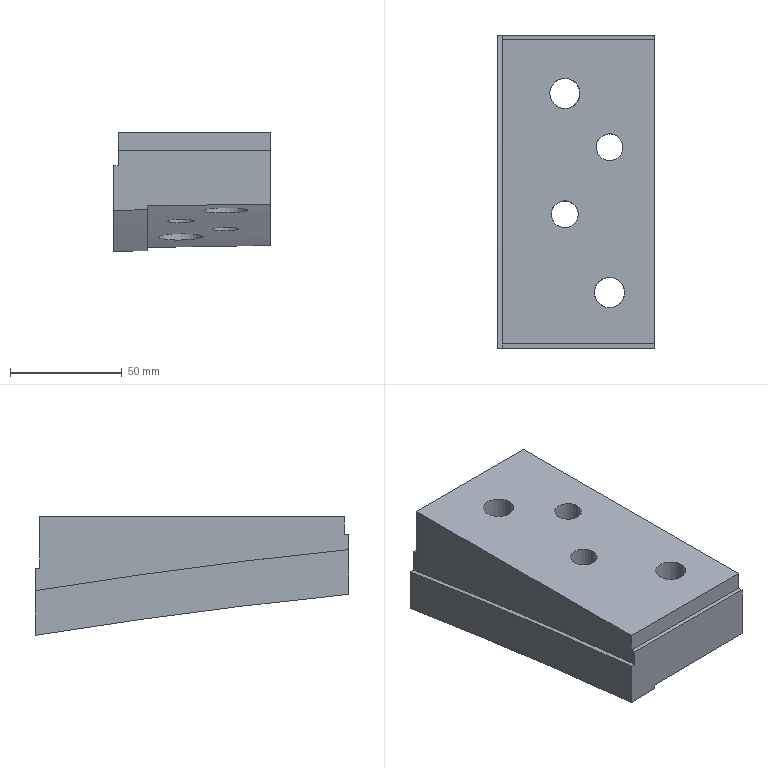Part | NX | features solid 2 | 1 solid | 22 faces | box 70.007 x 140 x 53.086 mm | volume 363707 mm3 | plane 11 | cylinder 6 | spline 5 | commonest cylinder face diameters 12 x2 13.5 x2 20 x2
STEP:
#1=CARTESIAN_POINT('',(-140.475,238.046,-39.891));
#2=VERTEX_POINT('',#1);
#3=CARTESIAN_POINT('',(-144.908,244.849,-40.783));
#4=CARTESIAN_POINT('',(-139.451,238.369,-39.899));
#5=CARTESIAN_POINT('',(-140.14,229.951,-38.967));
#6=CARTESIAN_POINT('',(-146.602,224.444,-38.492));
#7=CARTESIAN_POINT('',(-155.095,225.151,-38.667));
#8=CARTESIAN_POINT('',(-160.551,231.64,-39.426));
#9=CARTESIAN_POINT('',(-159.861,240.041,-40.4));
#10=CARTESIAN_POINT('',(-153.405,245.556,-40.999));
#11=CARTESIAN_POINT('',(-144.908,244.849,-40.783));
#12=CARTESIAN_POINT('',(-139.451,238.369,-39.899));
#13=CARTESIAN_POINT('',(-140.14,229.951,-38.967));
#14=B_SPLINE_CURVE_WITH_KNOTS('',3,(#3,#4,#5,#6,#7,#8,#9,#10,#11,#12,#13),.UNSPECIFIED.,.T.,.F.,(1,1,1,1,1,1,1,1,1,1,1,1,1,1,1),(-0.02352,-0.01568,-0.007841,0.,0.007841,0.01568,0.02352,0.03136,0.0392,0.04704,0.05488,0.06273,0.07057,0.07841,0.08625),.UNSPECIFIED.);
#15=EDGE_CURVE('',#2,#2,#14,.T.);
#16=ORIENTED_EDGE('',*,*,#15,.F.);
#17=EDGE_LOOP('',(#16));
#18=FACE_BOUND('',#17,.T.);
#19=CARTESIAN_POINT('',(-130.,210.,-36.981));
#20=VERTEX_POINT('',#19);
#21=CARTESIAN_POINT('',(-185.059,210.,-37.712));
#22=VERTEX_POINT('',#21);
#23=CARTESIAN_POINT('',(-130.,210.,-36.981));
#24=CARTESIAN_POINT('',(-148.354,210.,-37.164));
#25=CARTESIAN_POINT('',(-166.707,210.,-37.411));
#26=CARTESIAN_POINT('',(-185.059,210.,-37.712));
#27=B_SPLINE_CURVE_WITH_KNOTS('',3,(#23,#24,#25,#26),.UNSPECIFIED.,.F.,.F.,(4,4),(0.007875,0.06294),.UNSPECIFIED.);
#28=EDGE_CURVE('',#20,#22,#27,.T.);
#29=ORIENTED_EDGE('',*,*,#28,.T.);
#30=CARTESIAN_POINT('',(-185.051,350.,-56.35));
#31=VERTEX_POINT('',#30);
#32=CARTESIAN_POINT('',(-185.051,350.,-56.35));
#33=CARTESIAN_POINT('',(-185.051,347.11,-55.776));
#34=CARTESIAN_POINT('',(-185.051,341.347,-54.515));
#35=CARTESIAN_POINT('',(-185.052,332.644,-53.023));
#36=CARTESIAN_POINT('',(-185.052,323.905,-51.767));
#37=CARTESIAN_POINT('',(-185.053,312.248,-50.137));
#38=CARTESIAN_POINT('',(-185.054,297.648,-48.295));
#39=CARTESIAN_POINT('',(-185.055,280.134,-46.04));
#40=CARTESIAN_POINT('',(-185.056,262.622,-43.77));
#41=CARTESIAN_POINT('',(-185.057,239.283,-40.663));
#42=CARTESIAN_POINT('',(-185.058,221.738,-38.676));
#43=CARTESIAN_POINT('',(-185.059,210.,-37.712));
#44=B_SPLINE_CURVE_WITH_KNOTS('',3,(#32,#33,#34,#35,#36,#37,#38,#39,#40,#41,#42,#43),.UNSPECIFIED.,.F.,.F.,(4,1,1,1,1,1,1,1,1,4),(0.,0.008828,0.01766,0.02648,0.03531,0.05297,0.07062,0.08828,0.1059,0.1412),.UNSPECIFIED.);
#45=EDGE_CURVE('',#31,#22,#44,.T.);
#46=ORIENTED_EDGE('',*,*,#45,.F.);
#47=CARTESIAN_POINT('',(-130.,350.,-55.455));
#48=VERTEX_POINT('',#47);
#49=CARTESIAN_POINT('',(-185.051,350.,-56.35));
#50=CARTESIAN_POINT('',(-166.701,350.,-56.003));
#51=CARTESIAN_POINT('',(-148.351,350.,-55.701));
#52=CARTESIAN_POINT('',(-130.,350.,-55.455));
#53=B_SPLINE_CURVE_WITH_KNOTS('',3,(#49,#50,#51,#52),.UNSPECIFIED.,.F.,.F.,(4,4),(0.,0.05506),.UNSPECIFIED.);
#54=EDGE_CURVE('',#31,#48,#53,.T.);
#55=ORIENTED_EDGE('',*,*,#54,.T.);
#56=CARTESIAN_POINT('',(-130.,210.,-36.981));
#57=CARTESIAN_POINT('',(-130.,215.866,-37.48));
#58=CARTESIAN_POINT('',(-130.,227.593,-38.547));
#59=CARTESIAN_POINT('',(-130.,245.131,-40.566));
#60=CARTESIAN_POINT('',(-130.,262.629,-42.923));
#61=CARTESIAN_POINT('',(-130.,285.962,-46.042));
#62=CARTESIAN_POINT('',(-130.,306.401,-48.604));
#63=CARTESIAN_POINT('',(-130.,323.882,-51.062));
#64=CARTESIAN_POINT('',(-130.,332.626,-52.267));
#65=CARTESIAN_POINT('',(-130.,341.355,-53.576));
#66=CARTESIAN_POINT('',(-130.,347.112,-54.872));
#67=CARTESIAN_POINT('',(-130.,350.,-55.455));
#68=B_SPLINE_CURVE_WITH_KNOTS('',3,(#56,#57,#58,#59,#60,#61,#62,#63,#64,#65,#66,#67),.UNSPECIFIED.,.F.,.F.,(4,1,1,1,1,1,1,1,1,4),(0.1253,0.143,0.1607,0.1783,0.196,0.2313,0.2402,0.249,0.2578,0.2667),.UNSPECIFIED.);
#69=EDGE_CURVE('',#20,#48,#68,.T.);
#70=ORIENTED_EDGE('',*,*,#69,.F.);
#71=EDGE_LOOP('',(#29,#46,#55,#70));
#72=FACE_BOUND('',#71,.T.);
#73=CARTESIAN_POINT('',(-164.006,269.741,-44.336));
#74=VERTEX_POINT('',#73);
#75=CARTESIAN_POINT('',(-165.496,265.103,-43.749));
#76=CARTESIAN_POINT('',(-163.363,269.717,-44.324));
#77=CARTESIAN_POINT('',(-165.086,274.474,-44.975));
#78=CARTESIAN_POINT('',(-169.695,276.649,-45.33));
#79=CARTESIAN_POINT('',(-174.506,274.895,-45.18));
#80=CARTESIAN_POINT('',(-176.635,270.284,-44.613));
#81=CARTESIAN_POINT('',(-174.919,265.533,-43.962));
#82=CARTESIAN_POINT('',(-170.309,263.35,-43.598));
#83=CARTESIAN_POINT('',(-165.496,265.103,-43.749));
#84=CARTESIAN_POINT('',(-163.363,269.717,-44.324));
#85=CARTESIAN_POINT('',(-165.086,274.474,-44.975));
#86=B_SPLINE_CURVE_WITH_KNOTS('',3,(#75,#76,#77,#78,#79,#80,#81,#82,#83,#84,#85),.UNSPECIFIED.,.T.,.F.,(1,1,1,1,1,1,1,1,1,1,1,1,1,1,1),(-0.01413,-0.009418,-0.004709,0.,0.004709,0.009418,0.01413,0.01884,0.02355,0.02825,0.03296,0.03767,0.04238,0.04709,0.0518),.UNSPECIFIED.);
#87=EDGE_CURVE('',#74,#74,#86,.T.);
#88=ORIENTED_EDGE('',*,*,#87,.T.);
#89=EDGE_LOOP('',(#88));
#90=FACE_BOUND('',#89,.T.);
#91=CARTESIAN_POINT('',(-144.006,299.738,-47.966));
#92=VERTEX_POINT('',#91);
#93=CARTESIAN_POINT('',(-145.498,295.102,-47.38));
#94=CARTESIAN_POINT('',(-143.363,299.714,-47.955));
#95=CARTESIAN_POINT('',(-145.085,304.473,-48.594));
#96=CARTESIAN_POINT('',(-149.694,306.649,-48.931));
#97=CARTESIAN_POINT('',(-154.504,304.896,-48.766));
#98=CARTESIAN_POINT('',(-156.635,300.288,-48.198));
#99=CARTESIAN_POINT('',(-154.921,295.534,-47.558));
#100=CARTESIAN_POINT('',(-150.31,293.351,-47.213));
#101=CARTESIAN_POINT('',(-145.498,295.102,-47.38));
#102=CARTESIAN_POINT('',(-143.363,299.714,-47.955));
#103=CARTESIAN_POINT('',(-145.085,304.473,-48.594));
#104=B_SPLINE_CURVE_WITH_KNOTS('',3,(#93,#94,#95,#96,#97,#98,#99,#100,#101,#102,#103),.UNSPECIFIED.,.T.,.F.,(1,1,1,1,1,1,1,1,1,1,1,1,1,1,1),(-0.01413,-0.009417,-0.004709,0.,0.004709,0.009417,0.01413,0.01883,0.02354,0.02825,0.03296,0.03767,0.04238,0.04709,0.05179),.UNSPECIFIED.);
#105=EDGE_CURVE('',#92,#92,#104,.T.);
#106=ORIENTED_EDGE('',*,*,#105,.T.);
#107=EDGE_LOOP('',(#106));
#108=FACE_BOUND('',#107,.T.);
#109=CARTESIAN_POINT('',(-160.477,327.052,-51.854));
#110=VERTEX_POINT('',#109);
#111=CARTESIAN_POINT('',(-164.907,333.852,-52.912));
#112=CARTESIAN_POINT('',(-159.456,327.371,-51.876));
#113=CARTESIAN_POINT('',(-160.132,318.975,-50.708));
#114=CARTESIAN_POINT('',(-166.581,313.446,-50.044));
#115=CARTESIAN_POINT('',(-175.096,314.149,-50.262));
#116=CARTESIAN_POINT('',(-180.544,320.634,-51.233));
#117=CARTESIAN_POINT('',(-179.87,329.017,-52.412));
#118=CARTESIAN_POINT('',(-173.427,334.553,-53.166));
#119=CARTESIAN_POINT('',(-164.907,333.852,-52.912));
#120=CARTESIAN_POINT('',(-159.456,327.371,-51.876));
#121=CARTESIAN_POINT('',(-160.132,318.975,-50.708));
#122=B_SPLINE_CURVE_WITH_KNOTS('',3,(#111,#112,#113,#114,#115,#116,#117,#118,#119,#120,#121),.UNSPECIFIED.,.T.,.F.,(1,1,1,1,1,1,1,1,1,1,1,1,1,1,1),(-0.02356,-0.01571,-0.007854,0.,0.007854,0.01571,0.02356,0.03142,0.03927,0.04713,0.05498,0.06283,0.07069,0.07854,0.0864),.UNSPECIFIED.);
#123=EDGE_CURVE('',#110,#110,#122,.T.);
#124=ORIENTED_EDGE('',*,*,#123,.F.);
#125=EDGE_LOOP('',(#124));
#126=FACE_BOUND('',#125,.T.);
#127=CARTESIAN_POINT('',(-123.533,350.,-55.371));
#128=CARTESIAN_POINT('',(-123.808,346.762,-54.719));
#129=CARTESIAN_POINT('',(-124.343,340.897,-53.404));
#130=CARTESIAN_POINT('',(-124.7,332.345,-52.182));
#131=CARTESIAN_POINT('',(-125.265,323.079,-50.908));
#132=CARTESIAN_POINT('',(-125.708,313.774,-49.596));
#133=CARTESIAN_POINT('',(-126.223,303.143,-48.22));
#134=CARTESIAN_POINT('',(-126.653,293.837,-47.001));
#135=CARTESIAN_POINT('',(-127.126,283.202,-45.621));
#136=CARTESIAN_POINT('',(-127.551,273.894,-44.396));
#137=CARTESIAN_POINT('',(-127.996,263.256,-42.978));
#138=CARTESIAN_POINT('',(-128.475,253.944,-41.745));
#139=CARTESIAN_POINT('',(-128.584,243.308,-40.357));
#140=CARTESIAN_POINT('',(-128.994,233.989,-39.253));
#141=CARTESIAN_POINT('',(-129.319,223.335,-38.175));
#142=CARTESIAN_POINT('',(-129.645,215.772,-37.47));
#143=CARTESIAN_POINT('',(-129.599,210.889,-37.053));
#144=CARTESIAN_POINT('',(-129.587,210.,-36.977));
#145=CARTESIAN_POINT('',(-127.416,350.,-55.42));
#146=CARTESIAN_POINT('',(-127.695,346.762,-54.769));
#147=CARTESIAN_POINT('',(-128.237,340.897,-53.457));
#148=CARTESIAN_POINT('',(-128.607,332.345,-52.22));
#149=CARTESIAN_POINT('',(-129.185,323.079,-50.941));
#150=CARTESIAN_POINT('',(-129.64,313.774,-49.632));
#151=CARTESIAN_POINT('',(-130.168,303.143,-48.258));
#152=CARTESIAN_POINT('',(-130.609,293.837,-47.042));
#153=CARTESIAN_POINT('',(-131.094,283.202,-45.664));
#154=CARTESIAN_POINT('',(-131.53,273.894,-44.441));
#155=CARTESIAN_POINT('',(-131.986,263.256,-43.026));
#156=CARTESIAN_POINT('',(-132.475,253.944,-41.796));
#157=CARTESIAN_POINT('',(-132.598,243.308,-40.406));
#158=CARTESIAN_POINT('',(-133.016,233.989,-39.301));
#159=CARTESIAN_POINT('',(-133.352,223.335,-38.215));
#160=CARTESIAN_POINT('',(-133.683,215.772,-37.509));
#161=CARTESIAN_POINT('',(-133.643,210.889,-37.093));
#162=CARTESIAN_POINT('',(-133.632,210.,-37.017));
#163=CARTESIAN_POINT('',(-148.045,350.,-55.695));
#164=CARTESIAN_POINT('',(-148.346,346.762,-55.05));
#165=CARTESIAN_POINT('',(-148.925,340.897,-53.748));
#166=CARTESIAN_POINT('',(-149.367,332.345,-52.436));
#167=CARTESIAN_POINT('',(-150.012,323.079,-51.132));
#168=CARTESIAN_POINT('',(-150.53,313.774,-49.839));
#169=CARTESIAN_POINT('',(-151.127,303.143,-48.475));
#170=CARTESIAN_POINT('',(-151.627,293.837,-47.269));
#171=CARTESIAN_POINT('',(-152.178,283.202,-45.906));
#172=CARTESIAN_POINT('',(-152.669,273.894,-44.696));
#173=CARTESIAN_POINT('',(-153.189,263.256,-43.294));
#174=CARTESIAN_POINT('',(-153.727,253.944,-42.079));
#175=CARTESIAN_POINT('',(-153.924,243.308,-40.681));
#176=CARTESIAN_POINT('',(-154.388,233.989,-39.571));
#177=CARTESIAN_POINT('',(-154.777,223.335,-38.441));
#178=CARTESIAN_POINT('',(-155.141,215.772,-37.733));
#179=CARTESIAN_POINT('',(-155.132,210.889,-37.321));
#180=CARTESIAN_POINT('',(-155.126,210.,-37.246));
#181=CARTESIAN_POINT('',(-168.673,350.,-56.04));
#182=CARTESIAN_POINT('',(-168.997,346.762,-55.399));
#183=CARTESIAN_POINT('',(-169.612,340.897,-54.107));
#184=CARTESIAN_POINT('',(-170.127,332.345,-52.728));
#185=CARTESIAN_POINT('',(-170.837,323.079,-51.412));
#186=CARTESIAN_POINT('',(-171.419,313.774,-50.124));
#187=CARTESIAN_POINT('',(-172.085,303.143,-48.774));
#188=CARTESIAN_POINT('',(-172.643,293.837,-47.576));
#189=CARTESIAN_POINT('',(-173.26,283.202,-46.224));
#190=CARTESIAN_POINT('',(-173.807,273.894,-45.025));
#191=CARTESIAN_POINT('',(-174.389,263.256,-43.638));
#192=CARTESIAN_POINT('',(-174.978,253.944,-42.435));
#193=CARTESIAN_POINT('',(-175.247,243.308,-41.037));
#194=CARTESIAN_POINT('',(-175.758,233.989,-39.915));
#195=CARTESIAN_POINT('',(-176.2,223.335,-38.752));
#196=CARTESIAN_POINT('',(-176.596,215.772,-38.037));
#197=CARTESIAN_POINT('',(-176.618,210.889,-37.634));
#198=CARTESIAN_POINT('',(-176.618,210.,-37.561));
#199=CARTESIAN_POINT('',(-185.418,350.,-56.357));
#200=CARTESIAN_POINT('',(-185.759,346.762,-55.72));
#201=CARTESIAN_POINT('',(-186.405,340.897,-54.446));
#202=CARTESIAN_POINT('',(-186.978,332.345,-53.02));
#203=CARTESIAN_POINT('',(-187.743,323.079,-51.691));
#204=CARTESIAN_POINT('',(-188.375,313.774,-50.406));
#205=CARTESIAN_POINT('',(-189.097,303.143,-49.066));
#206=CARTESIAN_POINT('',(-189.703,293.837,-47.874));
#207=CARTESIAN_POINT('',(-190.374,283.202,-46.528));
#208=CARTESIAN_POINT('',(-190.966,273.894,-45.337));
#209=CARTESIAN_POINT('',(-191.599,263.256,-43.961));
#210=CARTESIAN_POINT('',(-192.227,253.944,-42.768));
#211=CARTESIAN_POINT('',(-192.556,243.308,-41.375));
#212=CARTESIAN_POINT('',(-193.106,233.989,-40.244));
#213=CARTESIAN_POINT('',(-193.591,223.335,-39.053));
#214=CARTESIAN_POINT('',(-194.013,215.772,-38.334));
#215=CARTESIAN_POINT('',(-194.06,210.889,-37.937));
#216=CARTESIAN_POINT('',(-194.065,210.,-37.865));
#217=B_SPLINE_SURFACE_WITH_KNOTS('',3,3,((#127,#128,#129,#130,#131,#132,#133,#134,#135,#136,#137,#138,#139,#140,#141,#142,#143,#144),(#145,#146,#147,#148,#149,#150,#151,#152,#153,#154,#155,#156,#157,#158,#159,#160,#161,#162),(#163,#164,#165,#166,#167,#168,#169,#170,#171,#172,#173,#174,#175,#176,#177,#178,#179,#180),(#181,#182,#183,#184,#185,#186,#187,#188,#189,#190,#191,#192,#193,#194,#195,#196,#197,#198),(#199,#200,#201,#202,#203,#204,#205,#206,#207,#208,#209,#210,#211,#212,#213,#214,#215,#216)),.UNSPECIFIED.,.F.,.F.,.F.,(4,1,4),(4,1,1,1,1,1,1,1,1,1,1,1,1,1,1,4),(0.6143,0.625,0.6709),(0.2465,0.2656,0.2812,0.2969,0.3203,0.3359,0.3594,0.375,0.3984,0.4141,0.4375,0.4531,0.4766,0.4922,0.5156,0.5208),.UNSPECIFIED.);
#218=ADVANCED_FACE('',(#18,#72,#90,#108,#126),#217,.F.);
#219=CARTESIAN_POINT('',(-130.,348.,-5.));
#220=VERTEX_POINT('',#219);
#221=CARTESIAN_POINT('',(-130.,348.,-28.));
#222=VERTEX_POINT('',#221);
#223=CARTESIAN_POINT('',(-130.,348.,-3.));
#224=DIRECTION('',(0.,0.,1.));
#225=VECTOR('',#224,1000.);
#226=LINE('',#223,#225);
#227=EDGE_CURVE('',#220,#222,#226,.F.);
#228=ORIENTED_EDGE('',*,*,#227,.F.);
#229=CARTESIAN_POINT('',(-130.,212.,-5.));
#230=VERTEX_POINT('',#229);
#231=CARTESIAN_POINT('',(-130.,0.,-5.));
#232=DIRECTION('',(0.,-1.,0.));
#233=VECTOR('',#232,1000.);
#234=LINE('',#231,#233);
#235=EDGE_CURVE('',#220,#230,#234,.T.);
#236=ORIENTED_EDGE('',*,*,#235,.T.);
#237=CARTESIAN_POINT('',(-130.,212.,-13.));
#238=VERTEX_POINT('',#237);
#239=CARTESIAN_POINT('',(-130.,212.,-3.));
#240=DIRECTION('',(0.,0.,-1.));
#241=VECTOR('',#240,1000.);
#242=LINE('',#239,#241);
#243=EDGE_CURVE('',#230,#238,#242,.T.);
#244=ORIENTED_EDGE('',*,*,#243,.T.);
#245=CARTESIAN_POINT('',(-130.,210.,-13.));
#246=VERTEX_POINT('',#245);
#247=CARTESIAN_POINT('',(-130.,210.,-13.));
#248=DIRECTION('',(0.,-1.,0.));
#249=VECTOR('',#248,1000.);
#250=LINE('',#247,#249);
#251=EDGE_CURVE('',#246,#238,#250,.F.);
#252=ORIENTED_EDGE('',*,*,#251,.F.);
#253=CARTESIAN_POINT('',(-130.,210.,2.));
#254=DIRECTION('',(0.,0.,1.));
#255=VECTOR('',#254,1000.);
#256=LINE('',#253,#255);
#257=EDGE_CURVE('',#20,#246,#256,.T.);
#258=ORIENTED_EDGE('',*,*,#257,.F.);
#259=ORIENTED_EDGE('',*,*,#69,.T.);
#260=CARTESIAN_POINT('',(-130.,350.,-28.));
#261=VERTEX_POINT('',#260);
#262=CARTESIAN_POINT('',(-130.,350.,-40.306));
#263=DIRECTION('',(0.,0.,-1.));
#264=VECTOR('',#263,1000.);
#265=LINE('',#262,#264);
#266=EDGE_CURVE('',#261,#48,#265,.T.);
#267=ORIENTED_EDGE('',*,*,#266,.F.);
#268=CARTESIAN_POINT('',(-130.,350.,-28.));
#269=DIRECTION('',(0.,-1.,0.));
#270=VECTOR('',#269,1000.);
#271=LINE('',#268,#270);
#272=EDGE_CURVE('',#261,#222,#271,.T.);
#273=ORIENTED_EDGE('',*,*,#272,.T.);
#274=EDGE_LOOP('',(#228,#236,#244,#252,#258,#259,#267,#273));
#275=FACE_BOUND('',#274,.T.);
#276=CARTESIAN_POINT('',(-130.,0.,2.));
#277=DIRECTION('',(-1.,0.,0.));
#278=DIRECTION('',(0.,0.,-1.));
#279=AXIS2_PLACEMENT_3D('',#276,#277,#278);
#280=PLANE('',#279);
#281=ADVANCED_FACE('',(#275),#280,.F.);
#282=CARTESIAN_POINT('',(-198.007,348.,-28.));
#283=VERTEX_POINT('',#282);
#284=CARTESIAN_POINT('',(-198.007,350.,-28.));
#285=VERTEX_POINT('',#284);
#286=CARTESIAN_POINT('',(-198.007,348.,-28.));
#287=CARTESIAN_POINT('',(-198.007,348.667,-28.));
#288=CARTESIAN_POINT('',(-198.007,349.333,-28.));
#289=CARTESIAN_POINT('',(-198.007,350.,-28.));
#290=B_SPLINE_CURVE_WITH_KNOTS('',3,(#286,#287,#288,#289),.UNSPECIFIED.,.F.,.F.,(4,4),(0.009782,0.01178),.UNSPECIFIED.);
#291=EDGE_CURVE('',#283,#285,#290,.T.);
#292=ORIENTED_EDGE('',*,*,#291,.T.);
#293=CARTESIAN_POINT('',(-198.007,350.,-38.086));
#294=VERTEX_POINT('',#293);
#295=CARTESIAN_POINT('',(-198.007,350.,201.914));
#296=DIRECTION('',(0.,0.,1.));
#297=VECTOR('',#296,1000.);
#298=LINE('',#295,#297);
#299=EDGE_CURVE('',#285,#294,#298,.F.);
#300=ORIENTED_EDGE('',*,*,#299,.T.);
#301=CARTESIAN_POINT('',(-198.,210.,-19.737));
#302=VERTEX_POINT('',#301);
#303=CARTESIAN_POINT('',(-198.007,350.,-38.086));
#304=CARTESIAN_POINT('',(-198.,303.542,-30.601));
#305=CARTESIAN_POINT('',(-198.,256.853,-24.469));
#306=CARTESIAN_POINT('',(-198.,210.,-19.737));
#307=B_SPLINE_CURVE_WITH_KNOTS('',3,(#303,#304,#305,#306),.UNSPECIFIED.,.F.,.F.,(4,4),(0.,0.5298),.UNSPECIFIED.);
#308=EDGE_CURVE('',#302,#294,#307,.F.);
#309=ORIENTED_EDGE('',*,*,#308,.F.);
#310=CARTESIAN_POINT('',(-198.,210.,-13.));
#311=VERTEX_POINT('',#310);
#312=CARTESIAN_POINT('',(-198.,210.,2.806));
#313=DIRECTION('',(0.,0.,1.));
#314=VECTOR('',#313,1000.);
#315=LINE('',#312,#314);
#316=EDGE_CURVE('',#302,#311,#315,.T.);
#317=ORIENTED_EDGE('',*,*,#316,.T.);
#318=CARTESIAN_POINT('',(-198.,212.,-13.));
#319=VERTEX_POINT('',#318);
#320=CARTESIAN_POINT('',(-198.,210.,-13.));
#321=DIRECTION('',(0.,-1.,0.));
#322=VECTOR('',#321,1000.);
#323=LINE('',#320,#322);
#324=EDGE_CURVE('',#311,#319,#323,.F.);
#325=ORIENTED_EDGE('',*,*,#324,.T.);
#326=CARTESIAN_POINT('',(-198.,212.,-5.));
#327=VERTEX_POINT('',#326);
#328=CARTESIAN_POINT('',(-198.,212.,-3.));
#329=DIRECTION('',(0.,0.,-1.));
#330=VECTOR('',#329,1000.);
#331=LINE('',#328,#330);
#332=EDGE_CURVE('',#327,#319,#331,.T.);
#333=ORIENTED_EDGE('',*,*,#332,.F.);
#334=CARTESIAN_POINT('',(-198.007,348.,-5.));
#335=VERTEX_POINT('',#334);
#336=CARTESIAN_POINT('',(-198.007,348.,-5.));
#337=CARTESIAN_POINT('',(-198.,302.667,-5.));
#338=CARTESIAN_POINT('',(-198.,257.333,-5.));
#339=CARTESIAN_POINT('',(-198.,212.,-5.));
#340=B_SPLINE_CURVE_WITH_KNOTS('',3,(#336,#337,#338,#339),.UNSPECIFIED.,.F.,.F.,(4,4),(0.3384,0.4744),.UNSPECIFIED.);
#341=EDGE_CURVE('',#335,#327,#340,.T.);
#342=ORIENTED_EDGE('',*,*,#341,.F.);
#343=CARTESIAN_POINT('',(-198.007,348.,-20.222));
#344=DIRECTION('',(0.,0.,1.));
#345=VECTOR('',#344,1000.);
#346=LINE('',#343,#345);
#347=EDGE_CURVE('',#283,#335,#346,.T.);
#348=ORIENTED_EDGE('',*,*,#347,.F.);
#349=EDGE_LOOP('',(#292,#300,#309,#317,#325,#333,#342,#348));
#350=FACE_BOUND('',#349,.T.);
#351=CARTESIAN_POINT('',(-198.,210.,-19.933));
#352=CARTESIAN_POINT('',(-198.,210.,13.225));
#353=CARTESIAN_POINT('',(-198.,256.853,-24.666));
#354=CARTESIAN_POINT('',(-198.,256.853,8.491));
#355=CARTESIAN_POINT('',(-198.,303.536,-30.797));
#356=CARTESIAN_POINT('',(-198.,303.536,2.361));
#357=CARTESIAN_POINT('',(-198.007,350.,-38.282));
#358=CARTESIAN_POINT('',(-198.007,350.,-5.125));
#359=B_SPLINE_SURFACE_WITH_KNOTS('',3,1,((#351,#352),(#353,#354),(#355,#356),(#357,#358)),.SURF_OF_LINEAR_EXTRUSION.,.F.,.F.,.F.,(4,4),(2,2),(0.4702,1.),(0.,1.),.PIECEWISE_BEZIER_KNOTS.);
#360=ADVANCED_FACE('',(#350),#359,.F.);
#361=CARTESIAN_POINT('',(-176.75,324.,-5.));
#362=VERTEX_POINT('',#361);
#363=CARTESIAN_POINT('',(-170.,324.,-5.));
#364=DIRECTION('',(0.,0.,-1.));
#365=DIRECTION('',(-1.,0.,0.));
#366=AXIS2_PLACEMENT_3D('',#363,#364,#365);
#367=CIRCLE('',#366,6.75);
#368=EDGE_CURVE('',#362,#362,#367,.F.);
#369=ORIENTED_EDGE('',*,*,#368,.F.);
#370=EDGE_LOOP('',(#369));
#371=FACE_BOUND('',#370,.T.);
#372=CARTESIAN_POINT('',(-156.,300.,-5.));
#373=VERTEX_POINT('',#372);
#374=CARTESIAN_POINT('',(-150.,300.,-5.));
#375=DIRECTION('',(0.,0.,-1.));
#376=DIRECTION('',(-1.,0.,0.));
#377=AXIS2_PLACEMENT_3D('',#374,#375,#376);
#378=CIRCLE('',#377,6.);
#379=EDGE_CURVE('',#373,#373,#378,.F.);
#380=ORIENTED_EDGE('',*,*,#379,.F.);
#381=EDGE_LOOP('',(#380));
#382=FACE_BOUND('',#381,.T.);
#383=CARTESIAN_POINT('',(-176.,270.,-5.));
#384=VERTEX_POINT('',#383);
#385=CARTESIAN_POINT('',(-170.,270.,-5.));
#386=DIRECTION('',(0.,0.,-1.));
#387=DIRECTION('',(-1.,0.,0.));
#388=AXIS2_PLACEMENT_3D('',#385,#386,#387);
#389=CIRCLE('',#388,6.);
#390=EDGE_CURVE('',#384,#384,#389,.F.);
#391=ORIENTED_EDGE('',*,*,#390,.F.);
#392=EDGE_LOOP('',(#391));
#393=FACE_BOUND('',#392,.T.);
#394=CARTESIAN_POINT('',(-156.75,235.,-5.));
#395=VERTEX_POINT('',#394);
#396=CARTESIAN_POINT('',(-150.,235.,-5.));
#397=DIRECTION('',(0.,0.,-1.));
#398=DIRECTION('',(-1.,0.,0.));
#399=AXIS2_PLACEMENT_3D('',#396,#397,#398);
#400=CIRCLE('',#399,6.75);
#401=EDGE_CURVE('',#395,#395,#400,.F.);
#402=ORIENTED_EDGE('',*,*,#401,.F.);
#403=EDGE_LOOP('',(#402));
#404=FACE_BOUND('',#403,.T.);
#405=ORIENTED_EDGE('',*,*,#341,.T.);
#406=CARTESIAN_POINT('',(-198.,212.,-5.));
#407=DIRECTION('',(1.,0.,0.));
#408=VECTOR('',#407,1000.);
#409=LINE('',#406,#408);
#410=EDGE_CURVE('',#327,#230,#409,.T.);
#411=ORIENTED_EDGE('',*,*,#410,.T.);
#412=ORIENTED_EDGE('',*,*,#235,.F.);
#413=CARTESIAN_POINT('',(-130.,348.,-5.));
#414=DIRECTION('',(-1.,0.,0.));
#415=VECTOR('',#414,1000.);
#416=LINE('',#413,#415);
#417=EDGE_CURVE('',#220,#335,#416,.T.);
#418=ORIENTED_EDGE('',*,*,#417,.T.);
#419=EDGE_LOOP('',(#405,#411,#412,#418));
#420=FACE_BOUND('',#419,.T.);
#421=CARTESIAN_POINT('',(0.,0.,-5.));
#422=DIRECTION('',(0.,0.,1.));
#423=DIRECTION('',(-1.,0.,0.));
#424=AXIS2_PLACEMENT_3D('',#421,#422,#423);
#425=PLANE('',#424);
#426=ADVANCED_FACE('',(#371,#382,#393,#404,#420),#425,.T.);
#427=CARTESIAN_POINT('',(-198.,210.,-13.));
#428=DIRECTION('',(1.,0.,0.));
#429=VECTOR('',#428,1000.);
#430=LINE('',#427,#429);
#431=EDGE_CURVE('',#311,#246,#430,.T.);
#432=ORIENTED_EDGE('',*,*,#431,.F.);
#433=ORIENTED_EDGE('',*,*,#316,.F.);
#434=CARTESIAN_POINT('',(-200.,210.,-19.737));
#435=VERTEX_POINT('',#434);
#436=CARTESIAN_POINT('',(-200.,210.,-19.737));
#437=CARTESIAN_POINT('',(-199.333,210.,-19.737));
#438=CARTESIAN_POINT('',(-198.667,210.,-19.737));
#439=CARTESIAN_POINT('',(-198.,210.,-19.737));
#440=B_SPLINE_CURVE_WITH_KNOTS('',3,(#436,#437,#438,#439),.UNSPECIFIED.,.F.,.F.,(4,4),(0.00001231,0.002012),.UNSPECIFIED.);
#441=EDGE_CURVE('',#435,#302,#440,.T.);
#442=ORIENTED_EDGE('',*,*,#441,.F.);
#443=CARTESIAN_POINT('',(-200.,210.,-39.737));
#444=VERTEX_POINT('',#443);
#445=CARTESIAN_POINT('',(-200.,210.,-34.243));
#446=DIRECTION('',(0.,0.,1.));
#447=VECTOR('',#446,1000.);
#448=LINE('',#445,#447);
#449=EDGE_CURVE('',#435,#444,#448,.F.);
#450=ORIENTED_EDGE('',*,*,#449,.T.);
#451=CARTESIAN_POINT('',(-185.059,210.,-39.489));
#452=VERTEX_POINT('',#451);
#453=CARTESIAN_POINT('',(-200.,210.,-39.737));
#454=CARTESIAN_POINT('',(-195.02,210.,-39.651));
#455=CARTESIAN_POINT('',(-190.039,210.,-39.568));
#456=CARTESIAN_POINT('',(-185.059,210.,-39.489));
#457=B_SPLINE_CURVE_WITH_KNOTS('',3,(#453,#454,#455,#456),.UNSPECIFIED.,.F.,.F.,(4,4),(0.000111,0.01505),.UNSPECIFIED.);
#458=EDGE_CURVE('',#444,#452,#457,.T.);
#459=ORIENTED_EDGE('',*,*,#458,.T.);
#460=CARTESIAN_POINT('',(-185.059,210.,-115.));
#461=DIRECTION('',(0.,0.,-1.));
#462=VECTOR('',#461,1000.);
#463=LINE('',#460,#462);
#464=EDGE_CURVE('',#22,#452,#463,.T.);
#465=ORIENTED_EDGE('',*,*,#464,.F.);
#466=ORIENTED_EDGE('',*,*,#28,.F.);
#467=ORIENTED_EDGE('',*,*,#257,.T.);
#468=EDGE_LOOP('',(#432,#433,#442,#450,#459,#465,#466,#467));
#469=FACE_BOUND('',#468,.T.);
#470=CARTESIAN_POINT('',(130.,210.,-37.085));
#471=DIRECTION('',(0.,1.,0.));
#472=DIRECTION('',(0.,0.,1.));
#473=AXIS2_PLACEMENT_3D('',#470,#471,#472);
#474=PLANE('',#473);
#475=ADVANCED_FACE('',(#469),#474,.F.);
#476=CARTESIAN_POINT('',(-130.,350.,-28.));
#477=DIRECTION('',(-1.,0.,0.));
#478=VECTOR('',#477,1000.);
#479=LINE('',#476,#478);
#480=EDGE_CURVE('',#261,#285,#479,.T.);
#481=ORIENTED_EDGE('',*,*,#480,.F.);
#482=ORIENTED_EDGE('',*,*,#266,.T.);
#483=ORIENTED_EDGE('',*,*,#54,.F.);
#484=CARTESIAN_POINT('',(-185.051,350.,-57.827));
#485=VERTEX_POINT('',#484);
#486=CARTESIAN_POINT('',(-185.051,350.,-115.));
#487=DIRECTION('',(0.,0.,-1.));
#488=VECTOR('',#487,1000.);
#489=LINE('',#486,#488);
#490=EDGE_CURVE('',#31,#485,#489,.T.);
#491=ORIENTED_EDGE('',*,*,#490,.T.);
#492=CARTESIAN_POINT('',(-200.007,350.,-58.086));
#493=VERTEX_POINT('',#492);
#494=CARTESIAN_POINT('',(-200.007,350.,-58.086));
#495=CARTESIAN_POINT('',(-195.022,350.,-57.996));
#496=CARTESIAN_POINT('',(-190.036,350.,-57.909));
#497=CARTESIAN_POINT('',(-185.051,350.,-57.827));
#498=B_SPLINE_CURVE_WITH_KNOTS('',3,(#494,#495,#496,#497),.UNSPECIFIED.,.F.,.F.,(4,4),(0.0001123,0.01507),.UNSPECIFIED.);
#499=EDGE_CURVE('',#493,#485,#498,.T.);
#500=ORIENTED_EDGE('',*,*,#499,.F.);
#501=CARTESIAN_POINT('',(-200.007,350.,-38.086));
#502=VERTEX_POINT('',#501);
#503=CARTESIAN_POINT('',(-200.007,350.,-36.84));
#504=DIRECTION('',(0.,0.,1.));
#505=VECTOR('',#504,1000.);
#506=LINE('',#503,#505);
#507=EDGE_CURVE('',#502,#493,#506,.F.);
#508=ORIENTED_EDGE('',*,*,#507,.F.);
#509=CARTESIAN_POINT('',(-198.007,350.,-38.086));
#510=CARTESIAN_POINT('',(-198.674,350.,-38.086));
#511=CARTESIAN_POINT('',(-199.34,350.,-38.086));
#512=CARTESIAN_POINT('',(-200.007,350.,-38.086));
#513=B_SPLINE_CURVE_WITH_KNOTS('',3,(#509,#510,#511,#512),.UNSPECIFIED.,.F.,.F.,(4,4),(0.,1.),.UNSPECIFIED.);
#514=EDGE_CURVE('',#502,#294,#513,.F.);
#515=ORIENTED_EDGE('',*,*,#514,.T.);
#516=ORIENTED_EDGE('',*,*,#299,.F.);
#517=EDGE_LOOP('',(#481,#482,#483,#491,#500,#508,#515,#516));
#518=FACE_BOUND('',#517,.T.);
#519=CARTESIAN_POINT('',(440.921,350.,-40.306));
#520=DIRECTION('',(0.,1.,0.));
#521=DIRECTION('',(0.,0.,1.));
#522=AXIS2_PLACEMENT_3D('',#519,#520,#521);
#523=PLANE('',#522);
#524=ADVANCED_FACE('',(#518),#523,.T.);
#525=CARTESIAN_POINT('',(-200.,210.,-19.737));
#526=CARTESIAN_POINT('',(-200.,256.834,-24.467));
#527=CARTESIAN_POINT('',(-200.,303.526,-30.599));
#528=CARTESIAN_POINT('',(-200.007,350.,-38.086));
#529=B_SPLINE_CURVE_WITH_KNOTS('',3,(#525,#526,#527,#528),.UNSPECIFIED.,.F.,.F.,(4,4),(0.1254,0.2666),.UNSPECIFIED.);
#530=EDGE_CURVE('',#435,#502,#529,.T.);
#531=ORIENTED_EDGE('',*,*,#530,.T.);
#532=ORIENTED_EDGE('',*,*,#507,.T.);
#533=CARTESIAN_POINT('',(-200.,210.,-39.737));
#534=CARTESIAN_POINT('',(-200.,256.853,-44.47));
#535=CARTESIAN_POINT('',(-200.,303.536,-50.6));
#536=CARTESIAN_POINT('',(-200.007,350.,-58.086));
#537=B_SPLINE_CURVE_WITH_KNOTS('',3,(#533,#534,#535,#536),.UNSPECIFIED.,.F.,.F.,(4,4),(0.1885,0.3298),.UNSPECIFIED.);
#538=EDGE_CURVE('',#444,#493,#537,.T.);
#539=ORIENTED_EDGE('',*,*,#538,.F.);
#540=ORIENTED_EDGE('',*,*,#449,.F.);
#541=EDGE_LOOP('',(#531,#532,#539,#540));
#542=FACE_BOUND('',#541,.T.);
#543=CARTESIAN_POINT('',(-200.007,350.,-58.316));
#544=CARTESIAN_POINT('',(-200.007,350.,-19.506));
#545=CARTESIAN_POINT('',(-200.,303.333,-58.316));
#546=CARTESIAN_POINT('',(-200.,303.333,-19.506));
#547=CARTESIAN_POINT('',(-200.,256.667,-58.316));
#548=CARTESIAN_POINT('',(-200.,256.667,-19.506));
#549=CARTESIAN_POINT('',(-200.,210.,-58.316));
#550=CARTESIAN_POINT('',(-200.,210.,-19.506));
#551=B_SPLINE_SURFACE_WITH_KNOTS('',3,1,((#543,#544),(#545,#546),(#547,#548),(#549,#550)),.SURF_OF_LINEAR_EXTRUSION.,.F.,.F.,.F.,(4,4),(2,2),(0.7824,0.8605),(0.,1.),.PIECEWISE_BEZIER_KNOTS.);
#552=ADVANCED_FACE('',(#542),#551,.T.);
#553=ORIENTED_EDGE('',*,*,#538,.T.);
#554=ORIENTED_EDGE('',*,*,#499,.T.);
#555=CARTESIAN_POINT('',(-185.051,350.,-57.827));
#556=CARTESIAN_POINT('',(-185.053,303.529,-50.345));
#557=CARTESIAN_POINT('',(-185.056,256.828,-44.217));
#558=CARTESIAN_POINT('',(-185.059,210.,-39.489));
#559=B_SPLINE_CURVE_WITH_KNOTS('',3,(#555,#556,#557,#558),.UNSPECIFIED.,.F.,.F.,(4,4),(0.06841,0.2096),.UNSPECIFIED.);
#560=EDGE_CURVE('',#485,#452,#559,.T.);
#561=ORIENTED_EDGE('',*,*,#560,.T.);
#562=ORIENTED_EDGE('',*,*,#458,.F.);
#563=EDGE_LOOP('',(#553,#554,#561,#562));
#564=FACE_BOUND('',#563,.T.);
#565=CARTESIAN_POINT('',(-200.097,350.875,-58.229));
#566=CARTESIAN_POINT('',(-196.312,350.866,-58.159));
#567=CARTESIAN_POINT('',(-192.527,350.858,-58.091));
#568=CARTESIAN_POINT('',(-188.741,350.851,-58.025));
#569=CARTESIAN_POINT('',(-184.956,350.843,-57.961));
#570=CARTESIAN_POINT('',(-200.1,315.32,-52.488));
#571=CARTESIAN_POINT('',(-196.315,315.312,-52.419));
#572=CARTESIAN_POINT('',(-192.53,315.304,-52.352));
#573=CARTESIAN_POINT('',(-188.745,315.296,-52.287));
#574=CARTESIAN_POINT('',(-184.959,315.289,-52.224));
#575=CARTESIAN_POINT('',(-200.104,279.857,-47.48));
#576=CARTESIAN_POINT('',(-196.318,279.849,-47.412));
#577=CARTESIAN_POINT('',(-192.533,279.841,-47.347));
#578=CARTESIAN_POINT('',(-188.748,279.834,-47.283));
#579=CARTESIAN_POINT('',(-184.963,279.826,-47.221));
#580=CARTESIAN_POINT('',(-200.107,244.476,-43.209));
#581=CARTESIAN_POINT('',(-196.322,244.468,-43.142));
#582=CARTESIAN_POINT('',(-192.536,244.46,-43.077));
#583=CARTESIAN_POINT('',(-188.751,244.452,-43.014));
#584=CARTESIAN_POINT('',(-184.966,244.445,-42.952));
#585=CARTESIAN_POINT('',(-200.111,209.163,-39.654));
#586=CARTESIAN_POINT('',(-196.326,209.155,-39.588));
#587=CARTESIAN_POINT('',(-192.54,209.147,-39.524));
#588=CARTESIAN_POINT('',(-188.755,209.14,-39.461));
#589=CARTESIAN_POINT('',(-184.969,209.132,-39.4));
#590=B_SPLINE_SURFACE_WITH_KNOTS('',4,4,((#565,#566,#567,#568,#569),(#570,#571,#572,#573,#574),(#575,#576,#577,#578,#579),(#580,#581,#582,#583,#584),(#585,#586,#587,#588,#589)),.UNSPECIFIED.,.F.,.F.,.F.,(5,5),(5,5),(0.3047,0.5195),(0.5564,0.5748),.PIECEWISE_BEZIER_KNOTS.);
#591=ADVANCED_FACE('',(#564),#590,.F.);
#592=ORIENTED_EDGE('',*,*,#464,.T.);
#593=ORIENTED_EDGE('',*,*,#560,.F.);
#594=ORIENTED_EDGE('',*,*,#490,.F.);
#595=ORIENTED_EDGE('',*,*,#45,.T.);
#596=EDGE_LOOP('',(#592,#593,#594,#595));
#597=FACE_BOUND('',#596,.T.);
#598=CARTESIAN_POINT('',(-185.071,-2.633,-115.));
#599=DIRECTION('',(1.,-0.00005855,0.));
#600=DIRECTION('',(-0.00005855,-1.,0.));
#601=AXIS2_PLACEMENT_3D('',#598,#599,#600);
#602=PLANE('',#601);
#603=ADVANCED_FACE('',(#597),#602,.T.);
#604=ORIENTED_EDGE('',*,*,#441,.T.);
#605=ORIENTED_EDGE('',*,*,#308,.T.);
#606=ORIENTED_EDGE('',*,*,#514,.F.);
#607=ORIENTED_EDGE('',*,*,#530,.F.);
#608=EDGE_LOOP('',(#604,#605,#606,#607));
#609=FACE_BOUND('',#608,.T.);
#610=CARTESIAN_POINT('',(-198.,210.,-19.737));
#611=CARTESIAN_POINT('',(-198.,212.636,-20.003));
#612=CARTESIAN_POINT('',(-198.,215.272,-20.274));
#613=CARTESIAN_POINT('',(-198.,262.113,-25.164));
#614=CARTESIAN_POINT('',(-198.,306.156,-31.023));
#615=CARTESIAN_POINT('',(-198.007,350.,-38.086));
#616=CARTESIAN_POINT('',(-200.,210.,-19.737));
#617=CARTESIAN_POINT('',(-200.,212.636,-20.003));
#618=CARTESIAN_POINT('',(-200.,215.272,-20.274));
#619=CARTESIAN_POINT('',(-200.,262.113,-25.164));
#620=CARTESIAN_POINT('',(-200.,306.156,-31.023));
#621=CARTESIAN_POINT('',(-200.007,350.,-38.086));
#622=CARTESIAN_POINT('',(-200.012,210.,-19.737));
#623=CARTESIAN_POINT('',(-200.012,212.636,-20.003));
#624=CARTESIAN_POINT('',(-200.012,215.272,-20.274));
#625=CARTESIAN_POINT('',(-200.012,262.113,-25.164));
#626=CARTESIAN_POINT('',(-200.012,306.156,-31.023));
#627=CARTESIAN_POINT('',(-200.019,350.,-38.086));
#628=B_SPLINE_SURFACE_WITH_KNOTS('',1,3,((#610,#611,#612,#613,#614,#615),(#616,#617,#618,#619,#620,#621),(#622,#623,#624,#625,#626,#627)),.RULED_SURF.,.F.,.F.,.F.,(2,1,2),(4,2,4),(0.,1.,1.006),(0.4702,0.5,1.),.UNSPECIFIED.);
#629=ADVANCED_FACE('',(#609),#628,.F.);
#630=ORIENTED_EDGE('',*,*,#251,.T.);
#631=CARTESIAN_POINT('',(-198.,212.,-13.));
#632=DIRECTION('',(-1.,0.,0.));
#633=VECTOR('',#632,1000.);
#634=LINE('',#631,#633);
#635=EDGE_CURVE('',#319,#238,#634,.F.);
#636=ORIENTED_EDGE('',*,*,#635,.F.);
#637=ORIENTED_EDGE('',*,*,#324,.F.);
#638=ORIENTED_EDGE('',*,*,#431,.T.);
#639=EDGE_LOOP('',(#630,#636,#637,#638));
#640=FACE_BOUND('',#639,.T.);
#641=CARTESIAN_POINT('',(-198.,210.,-13.));
#642=DIRECTION('',(0.,0.,1.));
#643=DIRECTION('',(1.,0.,0.));
#644=AXIS2_PLACEMENT_3D('',#641,#642,#643);
#645=PLANE('',#644);
#646=ADVANCED_FACE('',(#640),#645,.T.);
#647=ORIENTED_EDGE('',*,*,#635,.T.);
#648=ORIENTED_EDGE('',*,*,#243,.F.);
#649=ORIENTED_EDGE('',*,*,#410,.F.);
#650=ORIENTED_EDGE('',*,*,#332,.T.);
#651=EDGE_LOOP('',(#647,#648,#649,#650));
#652=FACE_BOUND('',#651,.T.);
#653=CARTESIAN_POINT('',(-198.,212.,-3.));
#654=DIRECTION('',(0.,-1.,0.));
#655=DIRECTION('',(0.,0.,-1.));
#656=AXIS2_PLACEMENT_3D('',#653,#654,#655);
#657=PLANE('',#656);
#658=ADVANCED_FACE('',(#652),#657,.T.);
#659=CARTESIAN_POINT('',(-130.,348.,-28.));
#660=DIRECTION('',(-1.,0.,0.));
#661=VECTOR('',#660,1000.);
#662=LINE('',#659,#661);
#663=EDGE_CURVE('',#222,#283,#662,.T.);
#664=ORIENTED_EDGE('',*,*,#663,.T.);
#665=ORIENTED_EDGE('',*,*,#347,.T.);
#666=ORIENTED_EDGE('',*,*,#417,.F.);
#667=ORIENTED_EDGE('',*,*,#227,.T.);
#668=EDGE_LOOP('',(#664,#665,#666,#667));
#669=FACE_BOUND('',#668,.T.);
#670=CARTESIAN_POINT('',(-130.,348.,-3.));
#671=DIRECTION('',(0.,1.,0.));
#672=DIRECTION('',(-1.,0.,0.));
#673=AXIS2_PLACEMENT_3D('',#670,#671,#672);
#674=PLANE('',#673);
#675=ADVANCED_FACE('',(#669),#674,.T.);
#676=ORIENTED_EDGE('',*,*,#291,.F.);
#677=ORIENTED_EDGE('',*,*,#663,.F.);
#678=ORIENTED_EDGE('',*,*,#272,.F.);
#679=ORIENTED_EDGE('',*,*,#480,.T.);
#680=EDGE_LOOP('',(#676,#677,#678,#679));
#681=FACE_BOUND('',#680,.T.);
#682=CARTESIAN_POINT('',(-130.,350.,-28.));
#683=DIRECTION('',(0.,0.,-1.));
#684=DIRECTION('',(1.,0.,0.));
#685=AXIS2_PLACEMENT_3D('',#682,#683,#684);
#686=PLANE('',#685);
#687=ADVANCED_FACE('',(#681),#686,.F.);
#688=ORIENTED_EDGE('',*,*,#15,.T.);
#689=EDGE_LOOP('',(#688));
#690=FACE_BOUND('',#689,.T.);
#691=CARTESIAN_POINT('',(-150.,245.,-20.));
#692=VERTEX_POINT('',#691);
#693=CARTESIAN_POINT('',(-150.,235.,-20.));
#694=DIRECTION('',(0.,0.,1.));
#695=DIRECTION('',(0.,1.,0.));
#696=AXIS2_PLACEMENT_3D('',#693,#694,#695);
#697=CIRCLE('',#696,10.);
#698=EDGE_CURVE('',#692,#692,#697,.F.);
#699=ORIENTED_EDGE('',*,*,#698,.F.);
#700=EDGE_LOOP('',(#699));
#701=FACE_BOUND('',#700,.T.);
#702=CARTESIAN_POINT('',(-150.,235.,-130.));
#703=DIRECTION('',(0.,0.,1.));
#704=DIRECTION('',(1.,0.,0.));
#705=AXIS2_PLACEMENT_3D('',#702,#703,#704);
#706=CYLINDRICAL_SURFACE('',#705,10.);
#707=ADVANCED_FACE('',(#690,#701),#706,.F.);
#708=CARTESIAN_POINT('',(-150.,241.75,-20.));
#709=VERTEX_POINT('',#708);
#710=CARTESIAN_POINT('',(-150.,235.,-20.));
#711=DIRECTION('',(0.,0.,1.));
#712=DIRECTION('',(0.,1.,0.));
#713=AXIS2_PLACEMENT_3D('',#710,#711,#712);
#714=CIRCLE('',#713,6.75);
#715=EDGE_CURVE('',#709,#709,#714,.F.);
#716=ORIENTED_EDGE('',*,*,#715,.F.);
#717=EDGE_LOOP('',(#716));
#718=FACE_BOUND('',#717,.T.);
#719=ORIENTED_EDGE('',*,*,#698,.T.);
#720=EDGE_LOOP('',(#719));
#721=FACE_BOUND('',#720,.T.);
#722=CARTESIAN_POINT('',(-150.,235.,-20.));
#723=DIRECTION('',(0.,0.,-1.));
#724=DIRECTION('',(0.,1.,0.));
#725=AXIS2_PLACEMENT_3D('',#722,#723,#724);
#726=PLANE('',#725);
#727=ADVANCED_FACE('',(#718,#721),#726,.T.);
#728=ORIENTED_EDGE('',*,*,#401,.T.);
#729=EDGE_LOOP('',(#728));
#730=FACE_BOUND('',#729,.T.);
#731=ORIENTED_EDGE('',*,*,#715,.T.);
#732=EDGE_LOOP('',(#731));
#733=FACE_BOUND('',#732,.T.);
#734=CARTESIAN_POINT('',(-150.,235.,-105.));
#735=DIRECTION('',(0.,0.,1.));
#736=DIRECTION('',(1.,0.,0.));
#737=AXIS2_PLACEMENT_3D('',#734,#735,#736);
#738=CYLINDRICAL_SURFACE('',#737,6.75);
#739=ADVANCED_FACE('',(#730,#733),#738,.F.);
#740=ORIENTED_EDGE('',*,*,#87,.F.);
#741=EDGE_LOOP('',(#740));
#742=FACE_BOUND('',#741,.T.);
#743=ORIENTED_EDGE('',*,*,#390,.T.);
#744=EDGE_LOOP('',(#743));
#745=FACE_BOUND('',#744,.T.);
#746=CARTESIAN_POINT('',(-170.,270.,-205.));
#747=DIRECTION('',(0.,0.,1.));
#748=DIRECTION('',(1.,0.,0.));
#749=AXIS2_PLACEMENT_3D('',#746,#747,#748);
#750=CYLINDRICAL_SURFACE('',#749,6.);
#751=ADVANCED_FACE('',(#742,#745),#750,.F.);
#752=ORIENTED_EDGE('',*,*,#105,.F.);
#753=EDGE_LOOP('',(#752));
#754=FACE_BOUND('',#753,.T.);
#755=ORIENTED_EDGE('',*,*,#379,.T.);
#756=EDGE_LOOP('',(#755));
#757=FACE_BOUND('',#756,.T.);
#758=CARTESIAN_POINT('',(-150.,300.,-205.));
#759=DIRECTION('',(0.,0.,1.));
#760=DIRECTION('',(1.,0.,0.));
#761=AXIS2_PLACEMENT_3D('',#758,#759,#760);
#762=CYLINDRICAL_SURFACE('',#761,6.);
#763=ADVANCED_FACE('',(#754,#757),#762,.F.);
#764=ORIENTED_EDGE('',*,*,#123,.T.);
#765=EDGE_LOOP('',(#764));
#766=FACE_BOUND('',#765,.T.);
#767=CARTESIAN_POINT('',(-170.,334.,-20.));
#768=VERTEX_POINT('',#767);
#769=CARTESIAN_POINT('',(-170.,324.,-20.));
#770=DIRECTION('',(0.,0.,1.));
#771=DIRECTION('',(0.,1.,0.));
#772=AXIS2_PLACEMENT_3D('',#769,#770,#771);
#773=CIRCLE('',#772,10.);
#774=EDGE_CURVE('',#768,#768,#773,.F.);
#775=ORIENTED_EDGE('',*,*,#774,.F.);
#776=EDGE_LOOP('',(#775));
#777=FACE_BOUND('',#776,.T.);
#778=CARTESIAN_POINT('',(-170.,324.,-130.));
#779=DIRECTION('',(0.,0.,1.));
#780=DIRECTION('',(1.,0.,0.));
#781=AXIS2_PLACEMENT_3D('',#778,#779,#780);
#782=CYLINDRICAL_SURFACE('',#781,10.);
#783=ADVANCED_FACE('',(#766,#777),#782,.F.);
#784=CARTESIAN_POINT('',(-170.,330.75,-20.));
#785=VERTEX_POINT('',#784);
#786=CARTESIAN_POINT('',(-170.,324.,-20.));
#787=DIRECTION('',(0.,0.,1.));
#788=DIRECTION('',(0.,1.,0.));
#789=AXIS2_PLACEMENT_3D('',#786,#787,#788);
#790=CIRCLE('',#789,6.75);
#791=EDGE_CURVE('',#785,#785,#790,.F.);
#792=ORIENTED_EDGE('',*,*,#791,.F.);
#793=EDGE_LOOP('',(#792));
#794=FACE_BOUND('',#793,.T.);
#795=ORIENTED_EDGE('',*,*,#774,.T.);
#796=EDGE_LOOP('',(#795));
#797=FACE_BOUND('',#796,.T.);
#798=CARTESIAN_POINT('',(-170.,324.,-20.));
#799=DIRECTION('',(0.,0.,-1.));
#800=DIRECTION('',(0.,1.,0.));
#801=AXIS2_PLACEMENT_3D('',#798,#799,#800);
#802=PLANE('',#801);
#803=ADVANCED_FACE('',(#794,#797),#802,.T.);
#804=ORIENTED_EDGE('',*,*,#368,.T.);
#805=EDGE_LOOP('',(#804));
#806=FACE_BOUND('',#805,.T.);
#807=ORIENTED_EDGE('',*,*,#791,.T.);
#808=EDGE_LOOP('',(#807));
#809=FACE_BOUND('',#808,.T.);
#810=CARTESIAN_POINT('',(-170.,324.,-105.));
#811=DIRECTION('',(0.,0.,1.));
#812=DIRECTION('',(1.,0.,0.));
#813=AXIS2_PLACEMENT_3D('',#810,#811,#812);
#814=CYLINDRICAL_SURFACE('',#813,6.75);
#815=ADVANCED_FACE('',(#806,#809),#814,.F.);
#816=CLOSED_SHELL('',(#218,#281,#360,#426,#475,#524,#552,#591,#603,#629,#646,#658,#675,#687,#707,#727,#739,#751,#763,#783,#803,#815));
#817=MANIFOLD_SOLID_BREP('',#816);
#818=(LENGTH_UNIT()NAMED_UNIT(*)SI_UNIT(.MILLI.,.METRE.));
#819=UNCERTAINTY_MEASURE_WITH_UNIT(LENGTH_MEASURE(0.0508),#818,'','');
#820=(NAMED_UNIT(*)PLANE_ANGLE_UNIT()SI_UNIT($,.RADIAN.));
#821=(NAMED_UNIT(*)SI_UNIT($,.STERADIAN.)SOLID_ANGLE_UNIT());
#822=(GEOMETRIC_REPRESENTATION_CONTEXT(3)GLOBAL_UNCERTAINTY_ASSIGNED_CONTEXT((#819))GLOBAL_UNIT_ASSIGNED_CONTEXT((#818,#820,#821))REPRESENTATION_CONTEXT('',''));
#823=ADVANCED_BREP_SHAPE_REPRESENTATION('',(#817),#822);